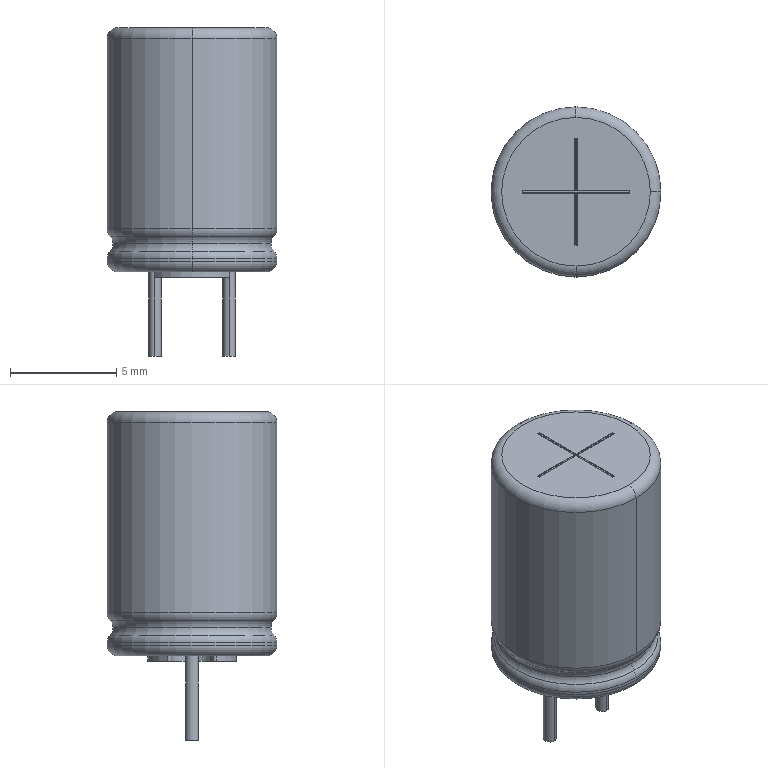Part | STEP file | RJ-USIO-V1_2-220411_270 | 1 solid | 69 faces | box 8 x 8 x 15.477 mm | volume 575.316 mm3 | cylinder 45 | torus 18 | plane 6 | commonest cylinder face diameters 0.02 x24 0.2 x6 8 x6 0.6 x4 2 x3 4.191 x1